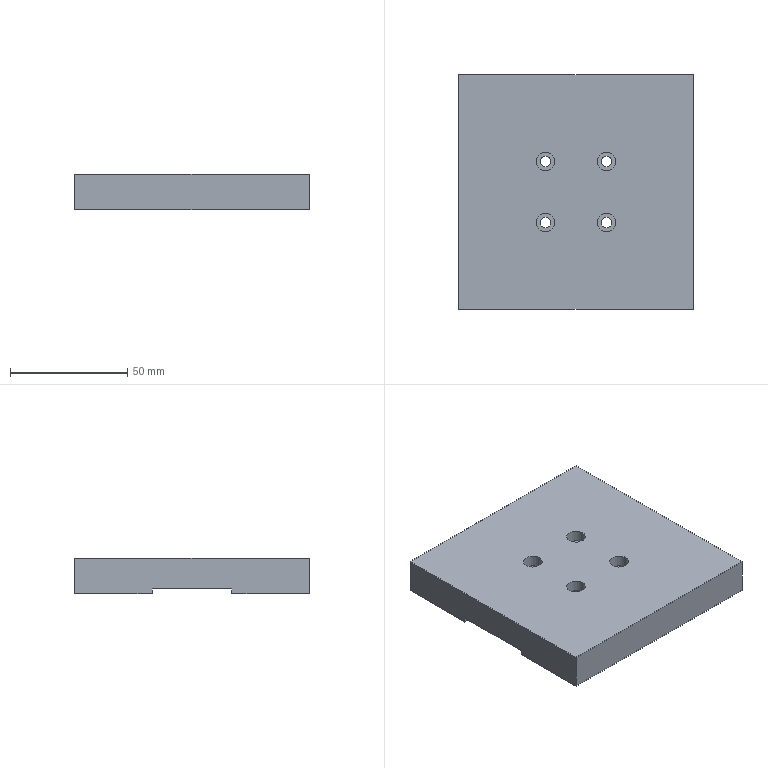Part | STEP file | Tube feed_id666_x_t | 1 solid | 22 faces | box 100 x 100 x 15 mm | volume 141686 mm3 | plane 14 | cylinder 8 | commonest cylinder face diameters 4.5 x4 8 x4